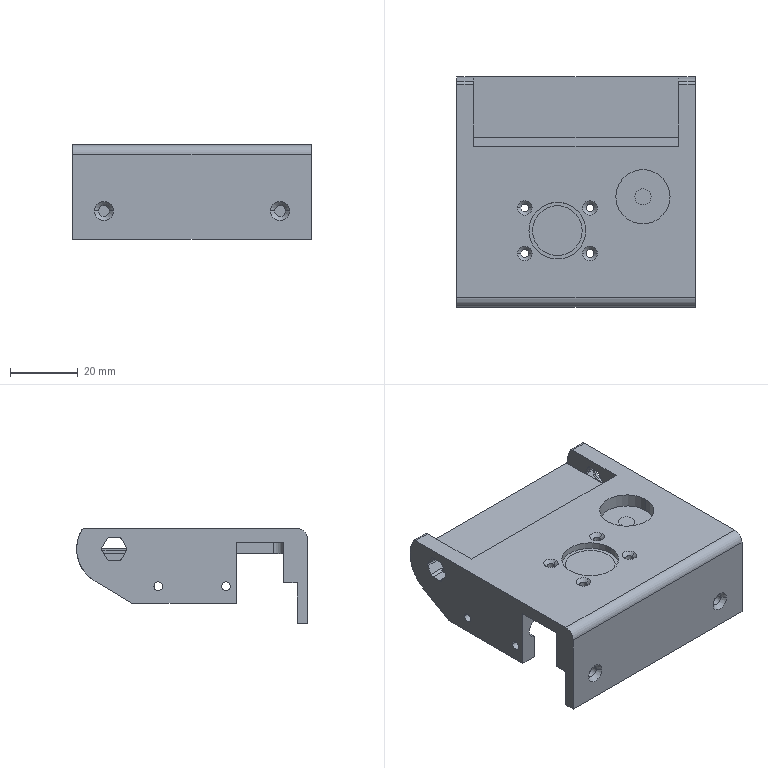NC program | NX | posted with a generic post | part box 70.5 x 68.1 x 28 mm
Lines 3639 to 4052 of 7250:
(FLOOR_WALL_1_COPY , TOOL : D10JING)
N7252 T11 M6
N7254 G54
N7256 G17 G0 G90 X39.1 Y35.981 B0. C0. S9500 M3
N7258 G43 Z30. H11
N7260 Z-4.5
N7262 G94 G1 Z-6. F1250.
N7264 X39.234 Y35.749
N7266 G3 X40.1 Y35.249 R1.
N7268 G1 X56.793
N7270 G3 X57.659 Y35.749 R1.
N7272 G1 X57.793 Y35.981
N7274 Z-4.5
N7276 G0 Z30.
N7278 X13.001 Y3.95
N7280 Z-19.
N7282 G1 Z-20.5
N7284 Y5.816
N7286 G3 X12.501 Y4.95 R1.
N7288 G1 Y40.25
N7290 X17.183
N7292 Y4.95
N7294 X21.864
N7296 Y40.25
N7298 X26.546
N7300 Y4.95
N7302 X31.227
N7304 Y40.25
N7306 X35.909
N7308 Y4.95
N7310 X39.
N7312 Y-24.75
N7314 X40.59
N7316 Y24.75
N7318 X45.272
N7320 Y-24.75
N7322 X49.953
N7324 Y24.75
N7326 X54.635
N7328 Y-24.75
N7330 X59.317
N7332 Y24.75
N7334 X63.998
N7336 Y-24.75
N7338 X68.68
N7340 Y24.75
N7342 G3 X67.814 Y24.25 R1.
N7344 G1 Z-19.
N7346 G0 Z30.
N7348 X73.998 Y24.518
N7350 Z-19.
N7352 G1 Z-20.5
N7354 X73.864 Y24.75
N7356 G3 X72.998 Y25.25 R1.
N7358 G1 X40.1
N7360 Y40.25
N7362 G3 X39.6 Y41.116 R1.
N7364 G1 X39.368 Y41.25
N7366 Z-19.
N7368 G0 Z30.
N7370 X12.732
N7372 Z-19.
N7374 G1 Z-20.5
N7376 X12.5 Y41.116
N7378 G3 X12. Y40.25 R1.
N7380 G1 Y4.95
N7382 G3 X12.5 Y4.084 R1.
N7384 G1 X13. Y3.795
N7386 Z-19.
N7388 G0 Z30.
N7390 X37.845 Y-24.25
N7392 Z-19.
N7394 G1 Z-20.5
N7396 X38.134 Y-24.75
N7398 G3 X39. Y-25.25 R1.
N7400 G1 X72.998
N7402 G3 X73.864 Y-24.75 R1.
N7404 G1 X73.998 Y-24.518
N7406 Z-19.
N7408 G0 Z30.
N7410 X9.232 Y41.25
N7412 Z-10.5
N7414 G1 Z-12.
N7416 X9. Y41.116
N7418 G3 X8.5 Y40.25 R1.
N7420 G1 Y-40.25
N7422 G3 X9. Y-41.116 R1.
N7424 G1 X9.232 Y-41.25
N7426 Z-10.5
N7428 G0 Z30.
N7430 X8.732 Y41.25
N7432 Z-10.5
N7434 G1 Z-12.
N7436 X8.5 Y41.116
N7438 G3 X8. Y40.25 R1.
N7440 G1 Y-40.25
N7442 G3 X8.5 Y-41.116 R1.
N7444 G1 X8.732 Y-41.25
N7446 Z-10.5
N7448 G0 Z30.
N7450 X22.6 Y-8.229
N7452 Z-23.9
N7454 G1 Y-8.4 Z-23.946
N7456 Y-2.6 Z-25.5
N7458 G2 X25.5 Y-5.497 R2.9
N7460 G1 Y-5.503
N7462 G2 X22.6 Y-8.4 R2.9
N7464 G1 Y-2.6
N7466 G3 X19.7 Y-5.497 R2.9
N7468 G1 Y-5.503
N7470 Z-24.
N7472 G0 Z30.
N7474 X23.218 Y-2.164
N7476 Z-23.9
N7478 G1 X22.861 Y-2.1 Z-23.997
N7480 X22.339 Z-24.137
N7482 X21.661 Y-2.222 Z-24.322
N7484 X21.02 Y-2.478 Z-24.506
N7486 X20.445 Y-2.857 Z-24.691
N7488 X19.957 Y-3.345 Z-24.876
N7490 X19.578 Y-3.92 Z-25.061
N7492 X19.322 Y-4.561 Z-25.245
N7494 X19.2 Y-5.239 Z-25.43
N7496 Y-5.5 Z-25.5
N7498 Y-5.504
N7500 G3 X22.604 Y-8.9 R3.4
N7502 X19.2 Y-5.5 R-3.4
N7504 G1 Z-24.
N7506 G0 Z30.
N7508 X13.001 Y-41.25
N7510 Z-22.5
N7512 G1 Z-24.
N7514 Y-39.384
N7516 G3 X12.501 Y-40.25 R1.
N7518 G1 Y4.45
N7520 X16.834
N7522 Y-24.75
N7524 X21.167
N7526 Y4.45
N7528 X25.5
N7530 Y-24.75
N7532 X29.834
N7534 Y4.45
N7536 X34.167
N7538 Y-24.75
N7540 X38.5
N7542 Y4.45
N7544 G3 X37.634 Y3.95 R1.
N7546 G1 Z-22.5
N7548 G0 Z30.
N7550 X15.268 Y-41.25
N7552 Z-22.5
N7554 G1 Z-24.
N7556 X15.5 Y-41.116
N7558 G3 X16. Y-40.25 R1.
N7560 G1 Y-25.25
N7562 X39.
N7564 Y4.95
N7566 X12.
N7568 Y-40.25
N7570 G3 X12.5 Y-41.116 R1.
N7572 G1 X12.732 Y-41.25
N7574 Z-22.5
N7576 G0 Z30.
N7578 X15. Y-29.519
N7580 Z-4.5
N7582 G1 Z-6.
N7584 X15.134 Y-29.751
N7586 G3 X16. Y-30.251 R1.
N7588 G1 X56.793
N7590 G3 X57.659 Y-29.751 R1.
N7592 G1 X57.793 Y-29.519
N7594 Z-4.5
N7596 G0 Z30.
N7598 M5
(ZLEVEL_PROFILE , TOOL : D6)
N7600 T06 M6
N7602 G54
N7604 G17 G0 G90 X38.091 Y-26.65 B0. C0. S9500 M3
N7606 G43 Z30. H6
N7608 Z-21.
N7610 G94 G1 X38.264 Y-26.95 F1600.
N7612 G3 X38.784 Y-27.25 R0.6
N7614 G1 X41.
N7616 Y-25.034
N7618 G3 X40.7 Y-24.514 R0.6
N7620 G1 X40.4 Y-24.341
N7622 G0 X38.091 Y-26.65 Z-21.5
N7624 G1 X38.264 Y-26.95
N7626 G3 X38.784 Y-27.25 R0.6
N7628 G1 X41.
N7630 Y-25.034
N7632 G3 X40.7 Y-24.514 R0.6
N7634 G1 X40.4 Y-24.341
N7636 G0 X38.091 Y-26.65 Z-22.
N7638 G1 X38.264 Y-26.95
N7640 G3 X38.784 Y-27.25 R0.6
N7642 G1 X41.
N7644 Y-25.034
N7646 G3 X40.7 Y-24.514 R0.6
N7648 G1 X40.4 Y-24.341
N7650 G0 X38.091 Y-26.65 Z-22.5
N7652 G1 X38.264 Y-26.95
N7654 G3 X38.784 Y-27.25 R0.6
N7656 G1 X41.
N7658 Y-25.034
N7660 G3 X40.7 Y-24.514 R0.6
N7662 G1 X40.4 Y-24.341
N7664 G0 X38.091 Y-26.65 Z-23.
N7666 G1 X38.264 Y-26.95
N7668 G3 X38.784 Y-27.25 R0.6
N7670 G1 X41.
N7672 Y-25.034
N7674 G3 X40.7 Y-24.514 R0.6
N7676 G1 X40.4 Y-24.341
N7678 G0 X38.091 Y-26.65 Z-23.5
N7680 G1 X38.264 Y-26.95
N7682 G3 X38.784 Y-27.25 R0.6
N7684 G1 X41.
N7686 Y-25.034
N7688 G3 X40.7 Y-24.514 R0.6
N7690 G1 X40.4 Y-24.341
N7692 G0 X38.091 Y-26.65 Z-24.
N7694 G1 X38.264 Y-26.95
N7696 G3 X38.784 Y-27.25 R0.6
N7698 G1 X41.
N7700 Y-25.034
N7702 G3 X40.7 Y-24.514 R0.6
N7704 G1 X40.4 Y-24.341
N7706 G0 Z30.
N7708 Y4.041
N7710 Z-21.
N7712 G1 X40.7 Y4.214
N7714 G3 X41. Y4.734 R0.6
N7716 G1 Y6.95
N7718 X38.784
N7720 G3 X38.264 Y6.65 R0.6
N7722 G1 X38.091 Y6.35
N7724 G0 X40.4 Y4.041 Z-21.5
N7726 G1 X40.7 Y4.214
N7728 G3 X41. Y4.734 R0.6
N7730 G1 Y6.95
N7732 X38.784
N7734 G3 X38.264 Y6.65 R0.6
N7736 G1 X38.091 Y6.35
N7738 G0 X40.4 Y4.041 Z-22.
N7740 G1 X40.7 Y4.214
N7742 G3 X41. Y4.734 R0.6
N7744 G1 Y6.95
N7746 X38.784
N7748 G3 X38.264 Y6.65 R0.6
N7750 G1 X38.091 Y6.35
N7752 G0 X40.4 Y4.041 Z-22.5
N7754 G1 X40.7 Y4.214
N7756 G3 X41. Y4.734 R0.6
N7758 G1 Y6.95
N7760 X38.784
N7762 G3 X38.264 Y6.65 R0.6
N7764 G1 X38.091 Y6.35
N7766 G0 X40.4 Y4.041 Z-23.
N7768 G1 X40.7 Y4.214
N7770 G3 X41. Y4.734 R0.6
N7772 G1 Y6.95
N7774 X38.784
N7776 G3 X38.264 Y6.65 R0.6
N7778 G1 X38.091 Y6.35
N7780 G0 X40.4 Y4.041 Z-23.5
N7782 G1 X40.7 Y4.214
N7784 G3 X41. Y4.734 R0.6
N7786 G1 Y6.95
N7788 X38.784
N7790 G3 X38.264 Y6.65 R0.6
N7792 G1 X38.091 Y6.35
N7794 G0 X40.4 Y4.041 Z-24.
N7796 G1 X40.7 Y4.214
N7798 G3 X41. Y4.734 R0.6
N7800 G1 Y6.95
N7802 X38.784
N7804 G3 X38.264 Y6.65 R0.6
N7806 G1 X38.091 Y6.35
N7808 G0 Z30.
N7810 X12.909
N7812 Z-21.
N7814 G1 X12.736 Y6.65
N7816 G3 X12.216 Y6.95 R0.6
N7818 G1 X10.
N7820 Y4.734
N7822 G3 X10.3 Y4.214 R0.6
N7824 G1 X10.6 Y4.041
N7826 G0 X12.909 Y6.35 Z-21.5
N7828 G1 X12.736 Y6.65
N7830 G3 X12.216 Y6.95 R0.6
N7832 G1 X10.
N7834 Y4.734
N7836 G3 X10.3 Y4.214 R0.6
N7838 G1 X10.6 Y4.041
N7840 G0 X12.909 Y6.35 Z-22.
N7842 G1 X12.736 Y6.65
N7844 G3 X12.216 Y6.95 R0.6
N7846 G1 X10.
N7848 Y4.734
N7850 G3 X10.3 Y4.214 R0.6
N7852 G1 X10.6 Y4.041
N7854 G0 X12.909 Y6.35 Z-22.5
N7856 G1 X12.736 Y6.65
N7858 G3 X12.216 Y6.95 R0.6
N7860 G1 X10.
N7862 Y4.734
N7864 G3 X10.3 Y4.214 R0.6
N7866 G1 X10.6 Y4.041
N7868 G0 X12.909 Y6.35 Z-23.
N7870 G1 X12.736 Y6.65
N7872 G3 X12.216 Y6.95 R0.6
N7874 G1 X10.
N7876 Y4.734
N7878 G3 X10.3 Y4.214 R0.6
N7880 G1 X10.6 Y4.041
N7882 G0 X12.909 Y6.35 Z-23.5
N7884 G1 X12.736 Y6.65
N7886 G3 X12.216 Y6.95 R0.6
N7888 G1 X10.
N7890 Y4.734
N7892 G3 X10.3 Y4.214 R0.6
N7894 G1 X10.6 Y4.041
N7896 G0 X12.909 Y6.35 Z-24.
N7898 G1 X12.736 Y6.65
N7900 G3 X12.216 Y6.95 R0.6
N7902 G1 X10.
N7904 Y4.734
N7906 G3 X10.3 Y4.214 R0.6
N7908 G1 X10.6 Y4.041
N7910 G0 Z30.
(ZLEVEL_PROFILE_COPY_1 , TOOL : D6)
N7912 X56.059 Y26.5
N7914 Z-20.94
N7916 G1 X55.886 Y26.8
N7918 G3 X55.366 Y27.1 R0.6
N7920 G1 X53.15
N7922 Y24.884
N7924 G3 X53.45 Y24.364 R0.6
N7926 G1 X53.75 Y24.191
N7928 G0 X56.059 Y26.5 Z-21.38
N7930 G1 X55.886 Y26.8
N7932 G3 X55.366 Y27.1 R0.6
N7934 G1 X53.15
N7936 Y24.884
N7938 G3 X53.45 Y24.364 R0.6
N7940 G1 X53.75 Y24.191
N7942 G0 X56.059 Y26.5 Z-21.82
N7944 G1 X55.886 Y26.8
N7946 G3 X55.366 Y27.1 R0.6
N7948 G1 X53.15
N7950 Y24.884
N7952 G3 X53.45 Y24.364 R0.6
N7954 G1 X53.75 Y24.191
N7956 G0 X56.059 Y26.5 Z-22.26
N7958 G1 X55.886 Y26.8
N7960 G3 X55.366 Y27.1 R0.6
N7962 G1 X53.15
N7964 Y24.884
N7966 G3 X53.45 Y24.364 R0.6
N7968 G1 X53.75 Y24.191
N7970 G0 X56.059 Y26.5 Z-22.7
N7972 G1 X55.886 Y26.8
N7974 G3 X55.366 Y27.1 R0.6
N7976 G1 X53.15
N7978 Y24.884
N7980 G3 X53.45 Y24.364 R0.6
N7982 G1 X53.75 Y24.191
N7984 G0 Z30.
N7986 Y-24.176
N7988 Z-20.94
N7990 G1 X53.45 Y-24.349
N7992 G3 X53.15 Y-24.869 R0.6
N7994 G1 Y-27.1
N7996 X55.368
N7998 G3 X55.888 Y-26.8 R0.6
N8000 G1 X56.061 Y-26.5
N8002 G0 X53.75 Y-24.176 Z-21.38
N8004 G1 X53.45 Y-24.349
N8006 G3 X53.15 Y-24.869 R0.6
N8008 G1 Y-27.1
N8010 X55.368
N8012 G3 X55.888 Y-26.8 R0.6
N8014 G1 X56.061 Y-26.5
N8016 G0 X53.75 Y-24.176 Z-21.82
N8018 G1 X53.45 Y-24.349
N8020 G3 X53.15 Y-24.869 R0.6
N8022 G1 Y-27.1
N8024 X55.368
N8026 G3 X55.888 Y-26.8 R0.6
N8028 G1 X56.061 Y-26.5
N8030 G0 X53.75 Y-24.176 Z-22.26
N8032 G1 X53.45 Y-24.349
N8034 G3 X53.15 Y-24.869 R0.6
N8036 G1 Y-27.1
N8038 X55.368
N8040 G3 X55.888 Y-26.8 R0.6
N8042 G1 X56.061 Y-26.5
N8044 G0 X53.75 Y-24.176 Z-22.7
N8046 G1 X53.45 Y-24.349
N8048 G3 X53.15 Y-24.869 R0.6
N8050 G1 Y-27.1
N8052 X55.368
N8054 G3 X55.888 Y-26.8 R0.6
N8056 G1 X56.061 Y-26.5
N8058 G0 Z30.
N8060 M5